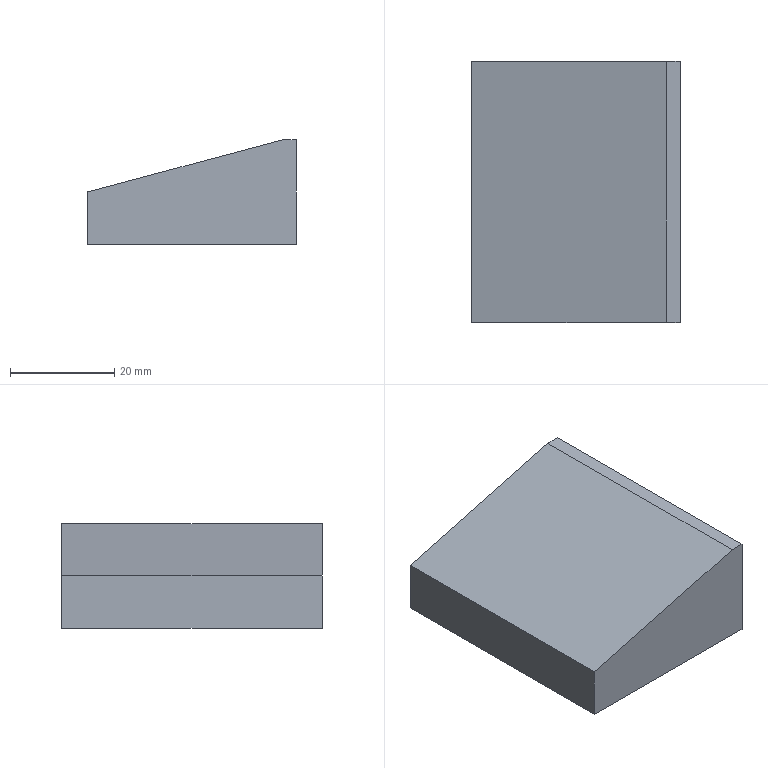Part | NX | features solid 2 | 1 solid | 7 faces | box 40 x 50 x 20 mm | volume 30670 mm3 | plane 7
STEP:
#1=CARTESIAN_POINT('',(-681.,-128.,-35.));
#2=VERTEX_POINT('',#1);
#3=CARTESIAN_POINT('',(-643.679,-128.,-25.));
#4=VERTEX_POINT('',#3);
#5=CARTESIAN_POINT('',(-683.5,-128.,-35.67));
#6=DIRECTION('',(0.9659,0.,0.2588));
#7=VECTOR('',#6,1000.);
#8=LINE('',#5,#7);
#9=EDGE_CURVE('',#2,#4,#8,.T.);
#10=ORIENTED_EDGE('',*,*,#9,.F.);
#11=CARTESIAN_POINT('',(-681.,-178.,-35.));
#12=VERTEX_POINT('',#11);
#13=CARTESIAN_POINT('',(-681.,-178.,-35.));
#14=DIRECTION('',(0.,1.,0.));
#15=VECTOR('',#14,1000.);
#16=LINE('',#13,#15);
#17=EDGE_CURVE('',#12,#2,#16,.T.);
#18=ORIENTED_EDGE('',*,*,#17,.F.);
#19=CARTESIAN_POINT('',(-643.679,-178.,-25.));
#20=VERTEX_POINT('',#19);
#21=CARTESIAN_POINT('',(-630.019,-178.,-21.34));
#22=DIRECTION('',(-0.9659,0.,-0.2588));
#23=VECTOR('',#22,1000.);
#24=LINE('',#21,#23);
#25=EDGE_CURVE('',#12,#20,#24,.F.);
#26=ORIENTED_EDGE('',*,*,#25,.T.);
#27=CARTESIAN_POINT('',(-643.679,-178.,-25.));
#28=DIRECTION('',(0.,1.,0.));
#29=VECTOR('',#28,1000.);
#30=LINE('',#27,#29);
#31=EDGE_CURVE('',#4,#20,#30,.F.);
#32=ORIENTED_EDGE('',*,*,#31,.F.);
#33=EDGE_LOOP('',(#10,#18,#26,#32));
#34=FACE_BOUND('',#33,.T.);
#35=CARTESIAN_POINT('',(-681.,-178.,-35.));
#36=DIRECTION('',(-0.2588,0.,0.9659));
#37=DIRECTION('',(-0.9659,0.,-0.2588));
#38=AXIS2_PLACEMENT_3D('',#35,#36,#37);
#39=PLANE('',#38);
#40=ADVANCED_FACE('',(#34),#39,.T.);
#41=CARTESIAN_POINT('',(-641.,-128.,-25.));
#42=VERTEX_POINT('',#41);
#43=CARTESIAN_POINT('',(-641.,-128.,-25.));
#44=DIRECTION('',(-1.,0.,0.));
#45=VECTOR('',#44,1000.);
#46=LINE('',#43,#45);
#47=EDGE_CURVE('',#4,#42,#46,.F.);
#48=ORIENTED_EDGE('',*,*,#47,.T.);
#49=CARTESIAN_POINT('',(-641.,-128.,-45.));
#50=VERTEX_POINT('',#49);
#51=CARTESIAN_POINT('',(-641.,-128.,-50.));
#52=DIRECTION('',(0.,0.,1.));
#53=VECTOR('',#52,1000.);
#54=LINE('',#51,#53);
#55=EDGE_CURVE('',#50,#42,#54,.T.);
#56=ORIENTED_EDGE('',*,*,#55,.F.);
#57=CARTESIAN_POINT('',(-681.,-128.,-45.));
#58=VERTEX_POINT('',#57);
#59=CARTESIAN_POINT('',(-681.,-128.,-45.));
#60=DIRECTION('',(-1.,0.,0.));
#61=VECTOR('',#60,1000.);
#62=LINE('',#59,#61);
#63=EDGE_CURVE('',#58,#50,#62,.F.);
#64=ORIENTED_EDGE('',*,*,#63,.F.);
#65=CARTESIAN_POINT('',(-681.,-128.,-45.));
#66=DIRECTION('',(0.,0.,1.));
#67=VECTOR('',#66,1000.);
#68=LINE('',#65,#67);
#69=EDGE_CURVE('',#58,#2,#68,.T.);
#70=ORIENTED_EDGE('',*,*,#69,.T.);
#71=ORIENTED_EDGE('',*,*,#9,.T.);
#72=EDGE_LOOP('',(#48,#56,#64,#70,#71));
#73=FACE_BOUND('',#72,.T.);
#74=CARTESIAN_POINT('',(-681.,-128.,-45.));
#75=DIRECTION('',(0.,-1.,0.));
#76=DIRECTION('',(0.,0.,-1.));
#77=AXIS2_PLACEMENT_3D('',#74,#75,#76);
#78=PLANE('',#77);
#79=ADVANCED_FACE('',(#73),#78,.F.);
#80=ORIENTED_EDGE('',*,*,#25,.F.);
#81=CARTESIAN_POINT('',(-681.,-178.,-45.));
#82=VERTEX_POINT('',#81);
#83=CARTESIAN_POINT('',(-681.,-178.,-55.));
#84=DIRECTION('',(0.,0.,-1.));
#85=VECTOR('',#84,1000.);
#86=LINE('',#83,#85);
#87=EDGE_CURVE('',#82,#12,#86,.F.);
#88=ORIENTED_EDGE('',*,*,#87,.F.);
#89=CARTESIAN_POINT('',(-641.,-178.,-45.));
#90=VERTEX_POINT('',#89);
#91=CARTESIAN_POINT('',(-681.,-178.,-45.));
#92=DIRECTION('',(1.,0.,0.));
#93=VECTOR('',#92,1000.);
#94=LINE('',#91,#93);
#95=EDGE_CURVE('',#82,#90,#94,.T.);
#96=ORIENTED_EDGE('',*,*,#95,.T.);
#97=CARTESIAN_POINT('',(-641.,-178.,-25.));
#98=VERTEX_POINT('',#97);
#99=CARTESIAN_POINT('',(-641.,-178.,-50.));
#100=DIRECTION('',(0.,0.,-1.));
#101=VECTOR('',#100,1000.);
#102=LINE('',#99,#101);
#103=EDGE_CURVE('',#90,#98,#102,.F.);
#104=ORIENTED_EDGE('',*,*,#103,.T.);
#105=CARTESIAN_POINT('',(-641.,-178.,-25.));
#106=DIRECTION('',(-1.,0.,0.));
#107=VECTOR('',#106,1000.);
#108=LINE('',#105,#107);
#109=EDGE_CURVE('',#20,#98,#108,.F.);
#110=ORIENTED_EDGE('',*,*,#109,.F.);
#111=EDGE_LOOP('',(#80,#88,#96,#104,#110));
#112=FACE_BOUND('',#111,.T.);
#113=CARTESIAN_POINT('',(-621.,-178.,-55.));
#114=DIRECTION('',(0.,1.,0.));
#115=DIRECTION('',(-1.,0.,0.));
#116=AXIS2_PLACEMENT_3D('',#113,#114,#115);
#117=PLANE('',#116);
#118=ADVANCED_FACE('',(#112),#117,.F.);
#119=ORIENTED_EDGE('',*,*,#103,.F.);
#120=CARTESIAN_POINT('',(-641.,-178.,-45.));
#121=DIRECTION('',(0.,-1.,0.));
#122=VECTOR('',#121,1000.);
#123=LINE('',#120,#122);
#124=EDGE_CURVE('',#90,#50,#123,.F.);
#125=ORIENTED_EDGE('',*,*,#124,.T.);
#126=ORIENTED_EDGE('',*,*,#55,.T.);
#127=CARTESIAN_POINT('',(-641.,-178.,-25.));
#128=DIRECTION('',(0.,1.,0.));
#129=VECTOR('',#128,1000.);
#130=LINE('',#127,#129);
#131=EDGE_CURVE('',#98,#42,#130,.T.);
#132=ORIENTED_EDGE('',*,*,#131,.F.);
#133=EDGE_LOOP('',(#119,#125,#126,#132));
#134=FACE_BOUND('',#133,.T.);
#135=CARTESIAN_POINT('',(-641.,-158.,-50.));
#136=DIRECTION('',(1.,0.,0.));
#137=DIRECTION('',(0.,1.,0.));
#138=AXIS2_PLACEMENT_3D('',#135,#136,#137);
#139=PLANE('',#138);
#140=ADVANCED_FACE('',(#134),#139,.T.);
#141=ORIENTED_EDGE('',*,*,#63,.T.);
#142=ORIENTED_EDGE('',*,*,#124,.F.);
#143=ORIENTED_EDGE('',*,*,#95,.F.);
#144=CARTESIAN_POINT('',(-681.,-178.,-45.));
#145=DIRECTION('',(0.,1.,0.));
#146=VECTOR('',#145,1000.);
#147=LINE('',#144,#146);
#148=EDGE_CURVE('',#58,#82,#147,.F.);
#149=ORIENTED_EDGE('',*,*,#148,.F.);
#150=EDGE_LOOP('',(#141,#142,#143,#149));
#151=FACE_BOUND('',#150,.T.);
#152=CARTESIAN_POINT('',(-681.,-178.,-45.));
#153=DIRECTION('',(0.,0.,1.));
#154=DIRECTION('',(1.,0.,0.));
#155=AXIS2_PLACEMENT_3D('',#152,#153,#154);
#156=PLANE('',#155);
#157=ADVANCED_FACE('',(#151),#156,.F.);
#158=ORIENTED_EDGE('',*,*,#148,.T.);
#159=ORIENTED_EDGE('',*,*,#87,.T.);
#160=ORIENTED_EDGE('',*,*,#17,.T.);
#161=ORIENTED_EDGE('',*,*,#69,.F.);
#162=EDGE_LOOP('',(#158,#159,#160,#161));
#163=FACE_BOUND('',#162,.T.);
#164=CARTESIAN_POINT('',(-681.,-153.5,-40.721));
#165=DIRECTION('',(-1.,0.,0.));
#166=DIRECTION('',(0.,1.,0.));
#167=AXIS2_PLACEMENT_3D('',#164,#165,#166);
#168=PLANE('',#167);
#169=ADVANCED_FACE('',(#163),#168,.T.);
#170=ORIENTED_EDGE('',*,*,#47,.F.);
#171=ORIENTED_EDGE('',*,*,#31,.T.);
#172=ORIENTED_EDGE('',*,*,#109,.T.);
#173=ORIENTED_EDGE('',*,*,#131,.T.);
#174=EDGE_LOOP('',(#170,#171,#172,#173));
#175=FACE_BOUND('',#174,.T.);
#176=CARTESIAN_POINT('',(-641.,-178.,-25.));
#177=DIRECTION('',(0.,0.,-1.));
#178=DIRECTION('',(0.,1.,0.));
#179=AXIS2_PLACEMENT_3D('',#176,#177,#178);
#180=PLANE('',#179);
#181=ADVANCED_FACE('',(#175),#180,.F.);
#182=CLOSED_SHELL('',(#40,#79,#118,#140,#157,#169,#181));
#183=MANIFOLD_SOLID_BREP('',#182);
#184=(LENGTH_UNIT()NAMED_UNIT(*)SI_UNIT(.MILLI.,.METRE.));
#185=UNCERTAINTY_MEASURE_WITH_UNIT(LENGTH_MEASURE(0.00001),#184,'','');
#186=(NAMED_UNIT(*)PLANE_ANGLE_UNIT()SI_UNIT($,.RADIAN.));
#187=(NAMED_UNIT(*)SI_UNIT($,.STERADIAN.)SOLID_ANGLE_UNIT());
#188=(GEOMETRIC_REPRESENTATION_CONTEXT(3)GLOBAL_UNCERTAINTY_ASSIGNED_CONTEXT((#185))GLOBAL_UNIT_ASSIGNED_CONTEXT((#184,#186,#187))REPRESENTATION_CONTEXT('',''));
#189=ADVANCED_BREP_SHAPE_REPRESENTATION('',(#183),#188);